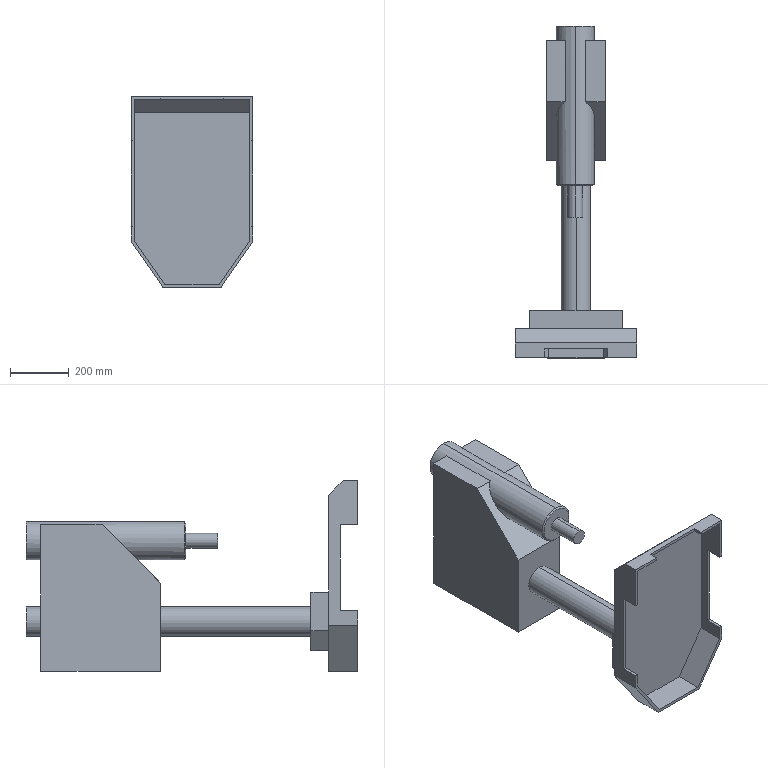Part | STEP file | 超升坡2-2 | 1 solid | 57 faces | box 415 x 1130 x 650 mm | volume 52548819 mm3 | plane 47 | cylinder 8 | cone 2 | commonest cylinder face diameters 100 x4 50 x2 130 x2